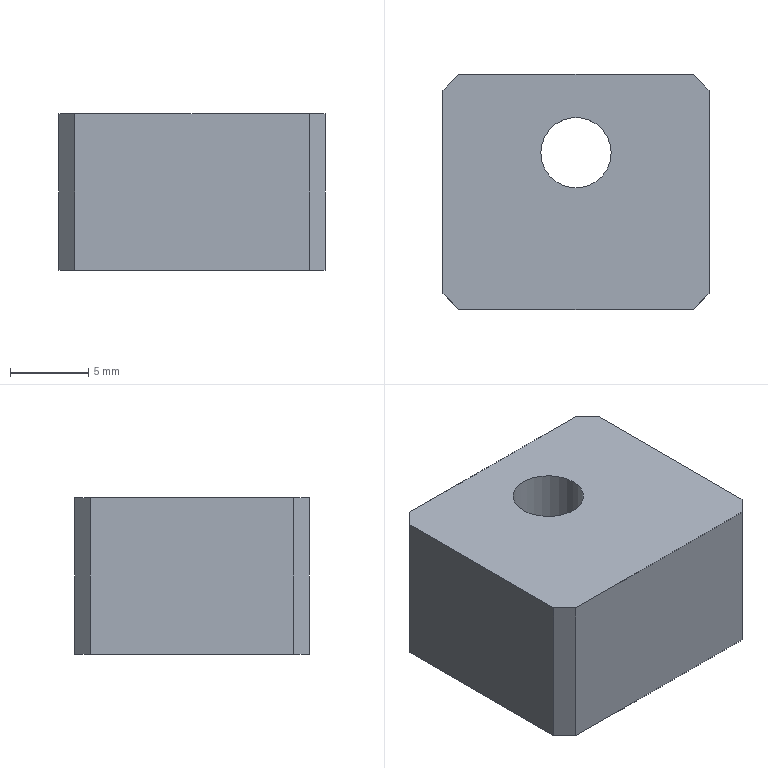Part | STEP file | 1_id906_x_t | 1 solid | 13 faces | box 17 x 15 x 10 mm | volume 2199 mm3 | plane 11 | cylinder 2 | commonest cylinder face diameters 4.5 x1 8 x1
STEP:
#1=CARTESIAN_POINT('',(0.,0.,0.));
#2=DIRECTION('',(0.,0.,1.));
#3=DIRECTION('',(1.,0.,0.));
#4=AXIS2_PLACEMENT_3D('',#1,#2,#3);
#5=CARTESIAN_POINT('',(628.275,227.376,-49.278));
#6=VERTEX_POINT('',#5);
#7=CARTESIAN_POINT('',(628.275,227.376,-59.278));
#8=VERTEX_POINT('',#7);
#9=CARTESIAN_POINT('',(628.275,227.376,-49.278));
#10=DIRECTION('',(0.,0.,-1.));
#11=VECTOR('',#10,1.);
#12=LINE('',#9,#11);
#13=CARTESIAN_POINT('',(627.275,228.376,-49.278));
#14=DIRECTION('',(0.7071,0.7071,0.));
#15=DIRECTION('',(0.,0.,1.));
#16=AXIS2_PLACEMENT_3D('',#13,#14,#15);
#17=PLANE('',#16);
#18=CARTESIAN_POINT('',(0.,1.414));
#19=DIRECTION('',(-1.,0.));
#20=VECTOR('',#19,1.);
#21=LINE('',#18,#20);
#22=(GEOMETRIC_REPRESENTATION_CONTEXT(2)PARAMETRIC_REPRESENTATION_CONTEXT()REPRESENTATION_CONTEXT('',''));
#23=DEFINITIONAL_REPRESENTATION('',(#21),#22);
#24=PCURVE('',#17,#23);
#25=CARTESIAN_POINT('',(643.275,227.376,-49.278));
#26=DIRECTION('',(0.,1.,0.));
#27=DIRECTION('',(-1.,0.,0.));
#28=AXIS2_PLACEMENT_3D('',#25,#26,#27);
#29=PLANE('',#28);
#30=CARTESIAN_POINT('',(15.,0.));
#31=DIRECTION('',(0.,-1.));
#32=VECTOR('',#31,1.);
#33=LINE('',#30,#32);
#34=(GEOMETRIC_REPRESENTATION_CONTEXT(2)PARAMETRIC_REPRESENTATION_CONTEXT()REPRESENTATION_CONTEXT('',''));
#35=DEFINITIONAL_REPRESENTATION('',(#33),#34);
#36=PCURVE('',#29,#35);
#37=SURFACE_CURVE('',#12,(#24,#36),.PCURVE_S1.);
#38=EDGE_CURVE('',#6,#8,#37,.T.);
#39=ORIENTED_EDGE('',*,*,#38,.F.);
#40=CARTESIAN_POINT('',(627.275,228.376,-49.278));
#41=VERTEX_POINT('',#40);
#42=CARTESIAN_POINT('',(627.275,228.376,-49.278));
#43=DIRECTION('',(0.7071,-0.7071,0.));
#44=VECTOR('',#43,1.);
#45=LINE('',#42,#44);
#46=CARTESIAN_POINT('',(0.,0.));
#47=DIRECTION('',(0.,1.));
#48=VECTOR('',#47,1.);
#49=LINE('',#46,#48);
#50=(GEOMETRIC_REPRESENTATION_CONTEXT(2)PARAMETRIC_REPRESENTATION_CONTEXT()REPRESENTATION_CONTEXT('',''));
#51=DEFINITIONAL_REPRESENTATION('',(#49),#50);
#52=PCURVE('',#17,#51);
#53=CARTESIAN_POINT('',(628.275,242.376,-49.278));
#54=DIRECTION('',(0.,0.,1.));
#55=DIRECTION('',(-1.,0.,0.));
#56=AXIS2_PLACEMENT_3D('',#53,#54,#55);
#57=PLANE('',#56);
#58=CARTESIAN_POINT('',(1.,14.));
#59=DIRECTION('',(-0.7071,0.7071));
#60=VECTOR('',#59,1.);
#61=LINE('',#58,#60);
#62=(GEOMETRIC_REPRESENTATION_CONTEXT(2)PARAMETRIC_REPRESENTATION_CONTEXT()REPRESENTATION_CONTEXT('',''));
#63=DEFINITIONAL_REPRESENTATION('',(#61),#62);
#64=PCURVE('',#57,#63);
#65=SURFACE_CURVE('',#45,(#52,#64),.PCURVE_S1.);
#66=EDGE_CURVE('',#41,#6,#65,.T.);
#67=ORIENTED_EDGE('',*,*,#66,.F.);
#68=CARTESIAN_POINT('',(627.275,228.376,-59.278));
#69=VERTEX_POINT('',#68);
#70=CARTESIAN_POINT('',(627.275,228.376,-59.278));
#71=DIRECTION('',(0.,0.,1.));
#72=VECTOR('',#71,1.);
#73=LINE('',#70,#72);
#74=CARTESIAN_POINT('',(-10.,0.));
#75=DIRECTION('',(1.,0.));
#76=VECTOR('',#75,1.);
#77=LINE('',#74,#76);
#78=(GEOMETRIC_REPRESENTATION_CONTEXT(2)PARAMETRIC_REPRESENTATION_CONTEXT()REPRESENTATION_CONTEXT('',''));
#79=DEFINITIONAL_REPRESENTATION('',(#77),#78);
#80=PCURVE('',#17,#79);
#81=CARTESIAN_POINT('',(627.275,227.376,-49.278));
#82=DIRECTION('',(1.,0.,0.));
#83=DIRECTION('',(0.,-1.,0.));
#84=AXIS2_PLACEMENT_3D('',#81,#82,#83);
#85=PLANE('',#84);
#86=CARTESIAN_POINT('',(-1.,10.));
#87=DIRECTION('',(0.,-1.));
#88=VECTOR('',#87,1.);
#89=LINE('',#86,#88);
#90=(GEOMETRIC_REPRESENTATION_CONTEXT(2)PARAMETRIC_REPRESENTATION_CONTEXT()REPRESENTATION_CONTEXT('',''));
#91=DEFINITIONAL_REPRESENTATION('',(#89),#90);
#92=PCURVE('',#85,#91);
#93=SURFACE_CURVE('',#73,(#80,#92),.PCURVE_S1.);
#94=EDGE_CURVE('',#69,#41,#93,.T.);
#95=ORIENTED_EDGE('',*,*,#94,.F.);
#96=CARTESIAN_POINT('',(628.275,227.376,-59.278));
#97=DIRECTION('',(-0.7071,0.7071,0.));
#98=VECTOR('',#97,1.);
#99=LINE('',#96,#98);
#100=CARTESIAN_POINT('',(-10.,1.414));
#101=DIRECTION('',(0.,-1.));
#102=VECTOR('',#101,1.);
#103=LINE('',#100,#102);
#104=(GEOMETRIC_REPRESENTATION_CONTEXT(2)PARAMETRIC_REPRESENTATION_CONTEXT()REPRESENTATION_CONTEXT('',''));
#105=DEFINITIONAL_REPRESENTATION('',(#103),#104);
#106=PCURVE('',#17,#105);
#107=CARTESIAN_POINT('',(628.275,242.376,-59.278));
#108=DIRECTION('',(0.,0.,1.));
#109=DIRECTION('',(-1.,0.,0.));
#110=AXIS2_PLACEMENT_3D('',#107,#108,#109);
#111=PLANE('',#110);
#112=CARTESIAN_POINT('',(0.,15.));
#113=DIRECTION('',(0.7071,-0.7071));
#114=VECTOR('',#113,1.);
#115=LINE('',#112,#114);
#116=(GEOMETRIC_REPRESENTATION_CONTEXT(2)PARAMETRIC_REPRESENTATION_CONTEXT()REPRESENTATION_CONTEXT('',''));
#117=DEFINITIONAL_REPRESENTATION('',(#115),#116);
#118=PCURVE('',#111,#117);
#119=SURFACE_CURVE('',#99,(#106,#118),.PCURVE_S1.);
#120=EDGE_CURVE('',#8,#69,#119,.T.);
#121=ORIENTED_EDGE('',*,*,#120,.F.);
#122=EDGE_LOOP('',(#39,#67,#95,#121));
#123=FACE_BOUND('',#122,.T.);
#124=ADVANCED_FACE('',(#123),#17,.F.);
#125=CARTESIAN_POINT('',(643.275,227.376,-59.278));
#126=VERTEX_POINT('',#125);
#127=CARTESIAN_POINT('',(628.275,227.376,-59.278));
#128=DIRECTION('',(1.,0.,0.));
#129=VECTOR('',#128,1.);
#130=LINE('',#127,#129);
#131=CARTESIAN_POINT('',(0.,15.));
#132=DIRECTION('',(-1.,0.));
#133=VECTOR('',#132,1.);
#134=LINE('',#131,#133);
#135=(GEOMETRIC_REPRESENTATION_CONTEXT(2)PARAMETRIC_REPRESENTATION_CONTEXT()REPRESENTATION_CONTEXT('',''));
#136=DEFINITIONAL_REPRESENTATION('',(#134),#135);
#137=PCURVE('',#111,#136);
#138=CARTESIAN_POINT('',(15.,-10.));
#139=DIRECTION('',(-1.,0.));
#140=VECTOR('',#139,1.);
#141=LINE('',#138,#140);
#142=(GEOMETRIC_REPRESENTATION_CONTEXT(2)PARAMETRIC_REPRESENTATION_CONTEXT()REPRESENTATION_CONTEXT('',''));
#143=DEFINITIONAL_REPRESENTATION('',(#141),#142);
#144=PCURVE('',#29,#143);
#145=SURFACE_CURVE('',#130,(#137,#144),.PCURVE_S1.);
#146=EDGE_CURVE('',#8,#126,#145,.T.);
#147=ORIENTED_EDGE('',*,*,#146,.F.);
#148=ORIENTED_EDGE('',*,*,#120,.T.);
#149=CARTESIAN_POINT('',(627.275,241.376,-59.278));
#150=VERTEX_POINT('',#149);
#151=CARTESIAN_POINT('',(627.275,241.376,-59.278));
#152=DIRECTION('',(0.,-1.,0.));
#153=VECTOR('',#152,1.);
#154=LINE('',#151,#153);
#155=CARTESIAN_POINT('',(1.,1.));
#156=DIRECTION('',(0.,1.));
#157=VECTOR('',#156,1.);
#158=LINE('',#155,#157);
#159=(GEOMETRIC_REPRESENTATION_CONTEXT(2)PARAMETRIC_REPRESENTATION_CONTEXT()REPRESENTATION_CONTEXT('',''));
#160=DEFINITIONAL_REPRESENTATION('',(#158),#159);
#161=PCURVE('',#111,#160);
#162=CARTESIAN_POINT('',(-14.,10.));
#163=DIRECTION('',(1.,0.));
#164=VECTOR('',#163,1.);
#165=LINE('',#162,#164);
#166=(GEOMETRIC_REPRESENTATION_CONTEXT(2)PARAMETRIC_REPRESENTATION_CONTEXT()REPRESENTATION_CONTEXT('',''));
#167=DEFINITIONAL_REPRESENTATION('',(#165),#166);
#168=PCURVE('',#85,#167);
#169=SURFACE_CURVE('',#154,(#161,#168),.PCURVE_S1.);
#170=EDGE_CURVE('',#150,#69,#169,.T.);
#171=ORIENTED_EDGE('',*,*,#170,.F.);
#172=CARTESIAN_POINT('',(628.275,242.376,-59.278));
#173=VERTEX_POINT('',#172);
#174=CARTESIAN_POINT('',(627.275,241.376,-59.278));
#175=DIRECTION('',(0.7071,0.7071,0.));
#176=VECTOR('',#175,1.);
#177=LINE('',#174,#176);
#178=CARTESIAN_POINT('',(1.,1.));
#179=DIRECTION('',(-0.7071,-0.7071));
#180=VECTOR('',#179,1.);
#181=LINE('',#178,#180);
#182=(GEOMETRIC_REPRESENTATION_CONTEXT(2)PARAMETRIC_REPRESENTATION_CONTEXT()REPRESENTATION_CONTEXT('',''));
#183=DEFINITIONAL_REPRESENTATION('',(#181),#182);
#184=PCURVE('',#111,#183);
#185=CARTESIAN_POINT('',(627.275,241.376,-49.278));
#186=DIRECTION('',(0.7071,-0.7071,0.));
#187=DIRECTION('',(0.7071,0.7071,0.));
#188=AXIS2_PLACEMENT_3D('',#185,#186,#187);
#189=PLANE('',#188);
#190=CARTESIAN_POINT('',(0.,-10.));
#191=DIRECTION('',(1.,0.));
#192=VECTOR('',#191,1.);
#193=LINE('',#190,#192);
#194=(GEOMETRIC_REPRESENTATION_CONTEXT(2)PARAMETRIC_REPRESENTATION_CONTEXT()REPRESENTATION_CONTEXT('',''));
#195=DEFINITIONAL_REPRESENTATION('',(#193),#194);
#196=PCURVE('',#189,#195);
#197=SURFACE_CURVE('',#177,(#184,#196),.PCURVE_S1.);
#198=EDGE_CURVE('',#150,#173,#197,.T.);
#199=ORIENTED_EDGE('',*,*,#198,.T.);
#200=CARTESIAN_POINT('',(643.275,242.376,-59.278));
#201=VERTEX_POINT('',#200);
#202=CARTESIAN_POINT('',(643.275,242.376,-59.278));
#203=DIRECTION('',(-1.,0.,0.));
#204=VECTOR('',#203,1.);
#205=LINE('',#202,#204);
#206=CARTESIAN_POINT('',(-15.,0.));
#207=DIRECTION('',(1.,0.));
#208=VECTOR('',#207,1.);
#209=LINE('',#206,#208);
#210=(GEOMETRIC_REPRESENTATION_CONTEXT(2)PARAMETRIC_REPRESENTATION_CONTEXT()REPRESENTATION_CONTEXT('',''));
#211=DEFINITIONAL_REPRESENTATION('',(#209),#210);
#212=PCURVE('',#111,#211);
#213=CARTESIAN_POINT('',(628.275,242.376,-49.278));
#214=DIRECTION('',(0.,-1.,0.));
#215=DIRECTION('',(0.,0.,1.));
#216=AXIS2_PLACEMENT_3D('',#213,#214,#215);
#217=PLANE('',#216);
#218=CARTESIAN_POINT('',(-10.,-15.));
#219=DIRECTION('',(0.,1.));
#220=VECTOR('',#219,1.);
#221=LINE('',#218,#220);
#222=(GEOMETRIC_REPRESENTATION_CONTEXT(2)PARAMETRIC_REPRESENTATION_CONTEXT()REPRESENTATION_CONTEXT('',''));
#223=DEFINITIONAL_REPRESENTATION('',(#221),#222);
#224=PCURVE('',#217,#223);
#225=SURFACE_CURVE('',#205,(#212,#224),.PCURVE_S1.);
#226=EDGE_CURVE('',#201,#173,#225,.T.);
#227=ORIENTED_EDGE('',*,*,#226,.F.);
#228=CARTESIAN_POINT('',(644.275,241.376,-59.278));
#229=VERTEX_POINT('',#228);
#230=CARTESIAN_POINT('',(643.275,242.376,-59.278));
#231=DIRECTION('',(0.7071,-0.7071,0.));
#232=VECTOR('',#231,1.);
#233=LINE('',#230,#232);
#234=CARTESIAN_POINT('',(-15.,0.));
#235=DIRECTION('',(-0.7071,0.7071));
#236=VECTOR('',#235,1.);
#237=LINE('',#234,#236);
#238=(GEOMETRIC_REPRESENTATION_CONTEXT(2)PARAMETRIC_REPRESENTATION_CONTEXT()REPRESENTATION_CONTEXT('',''));
#239=DEFINITIONAL_REPRESENTATION('',(#237),#238);
#240=PCURVE('',#111,#239);
#241=CARTESIAN_POINT('',(644.275,241.376,-49.278));
#242=DIRECTION('',(-0.7071,-0.7071,0.));
#243=DIRECTION('',(0.7071,-0.7071,0.));
#244=AXIS2_PLACEMENT_3D('',#241,#242,#243);
#245=PLANE('',#244);
#246=CARTESIAN_POINT('',(-1.414,-10.));
#247=DIRECTION('',(1.,0.));
#248=VECTOR('',#247,1.);
#249=LINE('',#246,#248);
#250=(GEOMETRIC_REPRESENTATION_CONTEXT(2)PARAMETRIC_REPRESENTATION_CONTEXT()REPRESENTATION_CONTEXT('',''));
#251=DEFINITIONAL_REPRESENTATION('',(#249),#250);
#252=PCURVE('',#245,#251);
#253=SURFACE_CURVE('',#233,(#240,#252),.PCURVE_S1.);
#254=EDGE_CURVE('',#201,#229,#253,.T.);
#255=ORIENTED_EDGE('',*,*,#254,.T.);
#256=CARTESIAN_POINT('',(644.275,228.376,-59.278));
#257=VERTEX_POINT('',#256);
#258=CARTESIAN_POINT('',(644.275,228.376,-59.278));
#259=DIRECTION('',(0.,1.,0.));
#260=VECTOR('',#259,1.);
#261=LINE('',#258,#260);
#262=CARTESIAN_POINT('',(-16.,14.));
#263=DIRECTION('',(0.,-1.));
#264=VECTOR('',#263,1.);
#265=LINE('',#262,#264);
#266=(GEOMETRIC_REPRESENTATION_CONTEXT(2)PARAMETRIC_REPRESENTATION_CONTEXT()REPRESENTATION_CONTEXT('',''));
#267=DEFINITIONAL_REPRESENTATION('',(#265),#266);
#268=PCURVE('',#111,#267);
#269=CARTESIAN_POINT('',(644.275,242.376,-49.278));
#270=DIRECTION('',(-1.,0.,0.));
#271=DIRECTION('',(0.,0.,-1.));
#272=AXIS2_PLACEMENT_3D('',#269,#270,#271);
#273=PLANE('',#272);
#274=CARTESIAN_POINT('',(10.,14.));
#275=DIRECTION('',(0.,-1.));
#276=VECTOR('',#275,1.);
#277=LINE('',#274,#276);
#278=(GEOMETRIC_REPRESENTATION_CONTEXT(2)PARAMETRIC_REPRESENTATION_CONTEXT()REPRESENTATION_CONTEXT('',''));
#279=DEFINITIONAL_REPRESENTATION('',(#277),#278);
#280=PCURVE('',#273,#279);
#281=SURFACE_CURVE('',#261,(#268,#280),.PCURVE_S1.);
#282=EDGE_CURVE('',#257,#229,#281,.T.);
#283=ORIENTED_EDGE('',*,*,#282,.F.);
#284=CARTESIAN_POINT('',(644.275,228.376,-59.278));
#285=DIRECTION('',(-0.7071,-0.7071,0.));
#286=VECTOR('',#285,1.);
#287=LINE('',#284,#286);
#288=CARTESIAN_POINT('',(-16.,14.));
#289=DIRECTION('',(0.7071,0.7071));
#290=VECTOR('',#289,1.);
#291=LINE('',#288,#290);
#292=(GEOMETRIC_REPRESENTATION_CONTEXT(2)PARAMETRIC_REPRESENTATION_CONTEXT()REPRESENTATION_CONTEXT('',''));
#293=DEFINITIONAL_REPRESENTATION('',(#291),#292);
#294=PCURVE('',#111,#293);
#295=CARTESIAN_POINT('',(643.275,227.376,-49.278));
#296=DIRECTION('',(-0.7071,0.7071,0.));
#297=DIRECTION('',(0.,0.,-1.));
#298=AXIS2_PLACEMENT_3D('',#295,#296,#297);
#299=PLANE('',#298);
#300=CARTESIAN_POINT('',(10.,-1.414));
#301=DIRECTION('',(0.,1.));
#302=VECTOR('',#301,1.);
#303=LINE('',#300,#302);
#304=(GEOMETRIC_REPRESENTATION_CONTEXT(2)PARAMETRIC_REPRESENTATION_CONTEXT()REPRESENTATION_CONTEXT('',''));
#305=DEFINITIONAL_REPRESENTATION('',(#303),#304);
#306=PCURVE('',#299,#305);
#307=SURFACE_CURVE('',#287,(#294,#306),.PCURVE_S1.);
#308=EDGE_CURVE('',#257,#126,#307,.T.);
#309=ORIENTED_EDGE('',*,*,#308,.T.);
#310=EDGE_LOOP('',(#147,#148,#171,#199,#227,#255,#283,#309));
#311=FACE_BOUND('',#310,.T.);
#312=CARTESIAN_POINT('',(631.775,237.376,-59.278));
#313=VERTEX_POINT('',#312);
#314=CARTESIAN_POINT('',(635.775,237.376,-59.278));
#315=DIRECTION('',(0.,0.,1.));
#316=DIRECTION('',(-1.,0.,0.));
#317=AXIS2_PLACEMENT_3D('',#314,#315,#316);
#318=CIRCLE('',#317,4.);
#319=CARTESIAN_POINT('',(-7.5,5.));
#320=DIRECTION('',(1.,0.));
#321=AXIS2_PLACEMENT_2D('',#319,#320);
#322=CIRCLE('',#321,4.);
#323=(GEOMETRIC_REPRESENTATION_CONTEXT(2)PARAMETRIC_REPRESENTATION_CONTEXT()REPRESENTATION_CONTEXT('',''));
#324=DEFINITIONAL_REPRESENTATION('',(#322),#323);
#325=PCURVE('',#111,#324);
#326=CARTESIAN_POINT('',(635.775,237.376,-54.278));
#327=DIRECTION('',(0.,0.,1.));
#328=DIRECTION('',(1.,0.,0.));
#329=AXIS2_PLACEMENT_3D('',#326,#327,#328);
#330=CYLINDRICAL_SURFACE('',#329,4.);
#331=CARTESIAN_POINT('',(3.142,-5.));
#332=DIRECTION('',(1.,0.));
#333=VECTOR('',#332,1.);
#334=LINE('',#331,#333);
#335=(GEOMETRIC_REPRESENTATION_CONTEXT(2)PARAMETRIC_REPRESENTATION_CONTEXT()REPRESENTATION_CONTEXT('',''));
#336=DEFINITIONAL_REPRESENTATION('',(#334),#335);
#337=PCURVE('',#330,#336);
#338=SURFACE_CURVE('',#318,(#325,#337),.PCURVE_S1.);
#339=EDGE_CURVE('',#313,#313,#338,.T.);
#340=ORIENTED_EDGE('',*,*,#339,.T.);
#341=EDGE_LOOP('',(#340));
#342=FACE_BOUND('',#341,.T.);
#343=ADVANCED_FACE('',(#311,#342),#111,.F.);
#344=CARTESIAN_POINT('',(643.275,227.376,-49.278));
#345=VERTEX_POINT('',#344);
#346=CARTESIAN_POINT('',(643.275,227.376,-59.278));
#347=DIRECTION('',(0.,0.,1.));
#348=VECTOR('',#347,1.);
#349=LINE('',#346,#348);
#350=CARTESIAN_POINT('',(10.,0.));
#351=DIRECTION('',(-1.,0.));
#352=VECTOR('',#351,1.);
#353=LINE('',#350,#352);
#354=(GEOMETRIC_REPRESENTATION_CONTEXT(2)PARAMETRIC_REPRESENTATION_CONTEXT()REPRESENTATION_CONTEXT('',''));
#355=DEFINITIONAL_REPRESENTATION('',(#353),#354);
#356=PCURVE('',#299,#355);
#357=CARTESIAN_POINT('',(0.,-10.));
#358=DIRECTION('',(0.,1.));
#359=VECTOR('',#358,1.);
#360=LINE('',#357,#359);
#361=(GEOMETRIC_REPRESENTATION_CONTEXT(2)PARAMETRIC_REPRESENTATION_CONTEXT()REPRESENTATION_CONTEXT('',''));
#362=DEFINITIONAL_REPRESENTATION('',(#360),#361);
#363=PCURVE('',#29,#362);
#364=SURFACE_CURVE('',#349,(#356,#363),.PCURVE_S1.);
#365=EDGE_CURVE('',#126,#345,#364,.T.);
#366=ORIENTED_EDGE('',*,*,#365,.F.);
#367=ORIENTED_EDGE('',*,*,#308,.F.);
#368=CARTESIAN_POINT('',(644.275,228.376,-49.278));
#369=VERTEX_POINT('',#368);
#370=CARTESIAN_POINT('',(644.275,228.376,-49.278));
#371=DIRECTION('',(0.,0.,-1.));
#372=VECTOR('',#371,1.);
#373=LINE('',#370,#372);
#374=CARTESIAN_POINT('',(0.,-1.414));
#375=DIRECTION('',(1.,0.));
#376=VECTOR('',#375,1.);
#377=LINE('',#374,#376);
#378=(GEOMETRIC_REPRESENTATION_CONTEXT(2)PARAMETRIC_REPRESENTATION_CONTEXT()REPRESENTATION_CONTEXT('',''));
#379=DEFINITIONAL_REPRESENTATION('',(#377),#378);
#380=PCURVE('',#299,#379);
#381=CARTESIAN_POINT('',(0.,14.));
#382=DIRECTION('',(1.,0.));
#383=VECTOR('',#382,1.);
#384=LINE('',#381,#383);
#385=(GEOMETRIC_REPRESENTATION_CONTEXT(2)PARAMETRIC_REPRESENTATION_CONTEXT()REPRESENTATION_CONTEXT('',''));
#386=DEFINITIONAL_REPRESENTATION('',(#384),#385);
#387=PCURVE('',#273,#386);
#388=SURFACE_CURVE('',#373,(#380,#387),.PCURVE_S1.);
#389=EDGE_CURVE('',#369,#257,#388,.T.);
#390=ORIENTED_EDGE('',*,*,#389,.F.);
#391=CARTESIAN_POINT('',(643.275,227.376,-49.278));
#392=DIRECTION('',(0.7071,0.7071,0.));
#393=VECTOR('',#392,1.);
#394=LINE('',#391,#393);
#395=CARTESIAN_POINT('',(0.,0.));
#396=DIRECTION('',(0.,-1.));
#397=VECTOR('',#396,1.);
#398=LINE('',#395,#397);
#399=(GEOMETRIC_REPRESENTATION_CONTEXT(2)PARAMETRIC_REPRESENTATION_CONTEXT()REPRESENTATION_CONTEXT('',''));
#400=DEFINITIONAL_REPRESENTATION('',(#398),#399);
#401=PCURVE('',#299,#400);
#402=CARTESIAN_POINT('',(-15.,15.));
#403=DIRECTION('',(-0.7071,-0.7071));
#404=VECTOR('',#403,1.);
#405=LINE('',#402,#404);
#406=(GEOMETRIC_REPRESENTATION_CONTEXT(2)PARAMETRIC_REPRESENTATION_CONTEXT()REPRESENTATION_CONTEXT('',''));
#407=DEFINITIONAL_REPRESENTATION('',(#405),#406);
#408=PCURVE('',#57,#407);
#409=SURFACE_CURVE('',#394,(#401,#408),.PCURVE_S1.);
#410=EDGE_CURVE('',#345,#369,#409,.T.);
#411=ORIENTED_EDGE('',*,*,#410,.F.);
#412=EDGE_LOOP('',(#366,#367,#390,#411));
#413=FACE_BOUND('',#412,.T.);
#414=ADVANCED_FACE('',(#413),#299,.F.);
#415=CARTESIAN_POINT('',(628.275,227.376,-49.278));
#416=DIRECTION('',(1.,0.,0.));
#417=VECTOR('',#416,1.);
#418=LINE('',#415,#417);
#419=CARTESIAN_POINT('',(0.,15.));
#420=DIRECTION('',(-1.,0.));
#421=VECTOR('',#420,1.);
#422=LINE('',#419,#421);
#423=(GEOMETRIC_REPRESENTATION_CONTEXT(2)PARAMETRIC_REPRESENTATION_CONTEXT()REPRESENTATION_CONTEXT('',''));
#424=DEFINITIONAL_REPRESENTATION('',(#422),#423);
#425=PCURVE('',#57,#424);
#426=CARTESIAN_POINT('',(15.,0.));
#427=DIRECTION('',(-1.,0.));
#428=VECTOR('',#427,1.);
#429=LINE('',#426,#428);
#430=(GEOMETRIC_REPRESENTATION_CONTEXT(2)PARAMETRIC_REPRESENTATION_CONTEXT()REPRESENTATION_CONTEXT('',''));
#431=DEFINITIONAL_REPRESENTATION('',(#429),#430);
#432=PCURVE('',#29,#431);
#433=SURFACE_CURVE('',#418,(#425,#432),.PCURVE_S1.);
#434=EDGE_CURVE('',#6,#345,#433,.T.);
#435=ORIENTED_EDGE('',*,*,#434,.T.);
#436=ORIENTED_EDGE('',*,*,#410,.T.);
#437=CARTESIAN_POINT('',(644.275,241.376,-49.278));
#438=VERTEX_POINT('',#437);
#439=CARTESIAN_POINT('',(644.275,228.376,-49.278));
#440=DIRECTION('',(0.,1.,0.));
#441=VECTOR('',#440,1.);
#442=LINE('',#439,#441);
#443=CARTESIAN_POINT('',(-16.,14.));
#444=DIRECTION('',(0.,-1.));
#445=VECTOR('',#444,1.);
#446=LINE('',#443,#445);
#447=(GEOMETRIC_REPRESENTATION_CONTEXT(2)PARAMETRIC_REPRESENTATION_CONTEXT()REPRESENTATION_CONTEXT('',''));
#448=DEFINITIONAL_REPRESENTATION('',(#446),#447);
#449=PCURVE('',#57,#448);
#450=CARTESIAN_POINT('',(0.,14.));
#451=DIRECTION('',(0.,-1.));
#452=VECTOR('',#451,1.);
#453=LINE('',#450,#452);
#454=(GEOMETRIC_REPRESENTATION_CONTEXT(2)PARAMETRIC_REPRESENTATION_CONTEXT()REPRESENTATION_CONTEXT('',''));
#455=DEFINITIONAL_REPRESENTATION('',(#453),#454);
#456=PCURVE('',#273,#455);
#457=SURFACE_CURVE('',#442,(#449,#456),.PCURVE_S1.);
#458=EDGE_CURVE('',#369,#438,#457,.T.);
#459=ORIENTED_EDGE('',*,*,#458,.T.);
#460=CARTESIAN_POINT('',(643.275,242.376,-49.278));
#461=VERTEX_POINT('',#460);
#462=CARTESIAN_POINT('',(644.275,241.376,-49.278));
#463=DIRECTION('',(-0.7071,0.7071,0.));
#464=VECTOR('',#463,1.);
#465=LINE('',#462,#464);
#466=CARTESIAN_POINT('',(-16.,1.));
#467=DIRECTION('',(0.7071,-0.7071));
#468=VECTOR('',#467,1.);
#469=LINE('',#466,#468);
#470=(GEOMETRIC_REPRESENTATION_CONTEXT(2)PARAMETRIC_REPRESENTATION_CONTEXT()REPRESENTATION_CONTEXT('',''));
#471=DEFINITIONAL_REPRESENTATION('',(#469),#470);
#472=PCURVE('',#57,#471);
#473=CARTESIAN_POINT('',(0.,0.));
#474=DIRECTION('',(-1.,0.));
#475=VECTOR('',#474,1.);
#476=LINE('',#473,#475);
#477=(GEOMETRIC_REPRESENTATION_CONTEXT(2)PARAMETRIC_REPRESENTATION_CONTEXT()REPRESENTATION_CONTEXT('',''));
#478=DEFINITIONAL_REPRESENTATION('',(#476),#477);
#479=PCURVE('',#245,#478);
#480=SURFACE_CURVE('',#465,(#472,#479),.PCURVE_S1.);
#481=EDGE_CURVE('',#438,#461,#480,.T.);
#482=ORIENTED_EDGE('',*,*,#481,.T.);
#483=CARTESIAN_POINT('',(628.275,242.376,-49.278));
#484=VERTEX_POINT('',#483);
#485=CARTESIAN_POINT('',(643.275,242.376,-49.278));
#486=DIRECTION('',(-1.,0.,0.));
#487=VECTOR('',#486,1.);
#488=LINE('',#485,#487);
#489=CARTESIAN_POINT('',(-15.,0.));
#490=DIRECTION('',(1.,0.));
#491=VECTOR('',#490,1.);
#492=LINE('',#489,#491);
#493=(GEOMETRIC_REPRESENTATION_CONTEXT(2)PARAMETRIC_REPRESENTATION_CONTEXT()REPRESENTATION_CONTEXT('',''));
#494=DEFINITIONAL_REPRESENTATION('',(#492),#493);
#495=PCURVE('',#57,#494);
#496=CARTESIAN_POINT('',(0.,-15.));
#497=DIRECTION('',(0.,1.));
#498=VECTOR('',#497,1.);
#499=LINE('',#496,#498);
#500=(GEOMETRIC_REPRESENTATION_CONTEXT(2)PARAMETRIC_REPRESENTATION_CONTEXT()REPRESENTATION_CONTEXT('',''));
#501=DEFINITIONAL_REPRESENTATION('',(#499),#500);
#502=PCURVE('',#217,#501);
#503=SURFACE_CURVE('',#488,(#495,#502),.PCURVE_S1.);
#504=EDGE_CURVE('',#461,#484,#503,.T.);
#505=ORIENTED_EDGE('',*,*,#504,.T.);
#506=CARTESIAN_POINT('',(627.275,241.376,-49.278));
#507=VERTEX_POINT('',#506);
#508=CARTESIAN_POINT('',(628.275,242.376,-49.278));
#509=DIRECTION('',(-0.7071,-0.7071,0.));
#510=VECTOR('',#509,1.);
#511=LINE('',#508,#510);
#512=CARTESIAN_POINT('',(0.,0.));
#513=DIRECTION('',(0.7071,0.7071));
#514=VECTOR('',#513,1.);
#515=LINE('',#512,#514);
#516=(GEOMETRIC_REPRESENTATION_CONTEXT(2)PARAMETRIC_REPRESENTATION_CONTEXT()REPRESENTATION_CONTEXT('',''));
#517=DEFINITIONAL_REPRESENTATION('',(#515),#516);
#518=PCURVE('',#57,#517);
#519=CARTESIAN_POINT('',(1.414,0.));
#520=DIRECTION('',(-1.,0.));
#521=VECTOR('',#520,1.);
#522=LINE('',#519,#521);
#523=(GEOMETRIC_REPRESENTATION_CONTEXT(2)PARAMETRIC_REPRESENTATION_CONTEXT()REPRESENTATION_CONTEXT('',''));
#524=DEFINITIONAL_REPRESENTATION('',(#522),#523);
#525=PCURVE('',#189,#524);
#526=SURFACE_CURVE('',#511,(#518,#525),.PCURVE_S1.);
#527=EDGE_CURVE('',#484,#507,#526,.T.);
#528=ORIENTED_EDGE('',*,*,#527,.T.);
#529=CARTESIAN_POINT('',(627.275,241.376,-49.278));
#530=DIRECTION('',(0.,-1.,0.));
#531=VECTOR('',#530,1.);
#532=LINE('',#529,#531);
#533=CARTESIAN_POINT('',(1.,1.));
#534=DIRECTION('',(0.,1.));
#535=VECTOR('',#534,1.);
#536=LINE('',#533,#535);
#537=(GEOMETRIC_REPRESENTATION_CONTEXT(2)PARAMETRIC_REPRESENTATION_CONTEXT()REPRESENTATION_CONTEXT('',''));
#538=DEFINITIONAL_REPRESENTATION('',(#536),#537);
#539=PCURVE('',#57,#538);
#540=CARTESIAN_POINT('',(-14.,0.));
#541=DIRECTION('',(1.,0.));
#542=VECTOR('',#541,1.);
#543=LINE('',#540,#542);
#544=(GEOMETRIC_REPRESENTATION_CONTEXT(2)PARAMETRIC_REPRESENTATION_CONTEXT()REPRESENTATION_CONTEXT('',''));
#545=DEFINITIONAL_REPRESENTATION('',(#543),#544);
#546=PCURVE('',#85,#545);
#547=SURFACE_CURVE('',#532,(#539,#546),.PCURVE_S1.);
#548=EDGE_CURVE('',#507,#41,#547,.T.);
#549=ORIENTED_EDGE('',*,*,#548,.T.);
#550=ORIENTED_EDGE('',*,*,#66,.T.);
#551=EDGE_LOOP('',(#435,#436,#459,#482,#505,#528,#549,#550));
#552=FACE_BOUND('',#551,.T.);
#553=CARTESIAN_POINT('',(638.025,237.376,-49.278));
#554=VERTEX_POINT('',#553);
#555=CARTESIAN_POINT('',(635.775,237.376,-49.278));
#556=DIRECTION('',(0.,0.,-1.));
#557=DIRECTION('',(1.,0.,0.));
#558=AXIS2_PLACEMENT_3D('',#555,#556,#557);
#559=CIRCLE('',#558,2.25);
#560=CARTESIAN_POINT('',(-9.75,5.));
#561=CARTESIAN_POINT('',(-9.75,8.897));
#562=CARTESIAN_POINT('',(-6.375,6.949));
#563=CARTESIAN_POINT('',(-3.,5.));
#564=CARTESIAN_POINT('',(-6.375,3.051));
#565=CARTESIAN_POINT('',(-9.75,1.103));
#566=CARTESIAN_POINT('',(-9.75,5.));
#567=(BOUNDED_CURVE()B_SPLINE_CURVE(2,(#560,#561,#562,#563,#564,#565,#566),.UNSPECIFIED.,.T.,.F.)B_SPLINE_CURVE_WITH_KNOTS((1,2,2,2,2,1),(-2.094,0.,2.094,4.189,6.283,8.378),.UNSPECIFIED.)CURVE()GEOMETRIC_REPRESENTATION_ITEM()RATIONAL_B_SPLINE_CURVE((1.,0.5,1.,0.5,1.,0.5,1.))REPRESENTATION_ITEM(''));
#568=(GEOMETRIC_REPRESENTATION_CONTEXT(2)PARAMETRIC_REPRESENTATION_CONTEXT()REPRESENTATION_CONTEXT('',''));
#569=DEFINITIONAL_REPRESENTATION('',(#567),#568);
#570=PCURVE('',#57,#569);
#571=CARTESIAN_POINT('',(635.775,237.376,-47.028));
#572=DIRECTION('',(0.,0.,1.));
#573=DIRECTION('',(1.,0.,0.));
#574=AXIS2_PLACEMENT_3D('',#571,#572,#573);
#575=CYLINDRICAL_SURFACE('',#574,2.25);
#576=CARTESIAN_POINT('',(6.283,-2.25));
#577=DIRECTION('',(-1.,0.));
#578=VECTOR('',#577,1.);
#579=LINE('',#576,#578);
#580=(GEOMETRIC_REPRESENTATION_CONTEXT(2)PARAMETRIC_REPRESENTATION_CONTEXT()REPRESENTATION_CONTEXT('',''));
#581=DEFINITIONAL_REPRESENTATION('',(#579),#580);
#582=PCURVE('',#575,#581);
#583=SURFACE_CURVE('',#559,(#570,#582),.PCURVE_S1.);
#584=EDGE_CURVE('',#554,#554,#583,.T.);
#585=ORIENTED_EDGE('',*,*,#584,.T.);
#586=EDGE_LOOP('',(#585));
#587=FACE_BOUND('',#586,.T.);
#588=ADVANCED_FACE('',(#552,#587),#57,.T.);
#589=CARTESIAN_POINT('',(627.275,241.376,-59.278));
#590=DIRECTION('',(0.,0.,1.));
#591=VECTOR('',#590,1.);
#592=LINE('',#589,#591);
#593=CARTESIAN_POINT('',(-14.,10.));
#594=DIRECTION('',(0.,-1.));
#595=VECTOR('',#594,1.);
#596=LINE('',#593,#595);
#597=(GEOMETRIC_REPRESENTATION_CONTEXT(2)PARAMETRIC_REPRESENTATION_CONTEXT()REPRESENTATION_CONTEXT('',''));
#598=DEFINITIONAL_REPRESENTATION('',(#596),#597);
#599=PCURVE('',#85,#598);
#600=CARTESIAN_POINT('',(0.,-10.));
#601=DIRECTION('',(0.,1.));
#602=VECTOR('',#601,1.);
#603=LINE('',#600,#602);
#604=(GEOMETRIC_REPRESENTATION_CONTEXT(2)PARAMETRIC_REPRESENTATION_CONTEXT()REPRESENTATION_CONTEXT('',''));
#605=DEFINITIONAL_REPRESENTATION('',(#603),#604);
#606=PCURVE('',#189,#605);
#607=SURFACE_CURVE('',#592,(#599,#606),.PCURVE_S1.);
#608=EDGE_CURVE('',#150,#507,#607,.T.);
#609=ORIENTED_EDGE('',*,*,#608,.F.);
#610=ORIENTED_EDGE('',*,*,#170,.T.);
#611=ORIENTED_EDGE('',*,*,#94,.T.);
#612=ORIENTED_EDGE('',*,*,#548,.F.);
#613=EDGE_LOOP('',(#609,#610,#611,#612));
#614=FACE_BOUND('',#613,.T.);
#615=ADVANCED_FACE('',(#614),#85,.F.);
#616=CARTESIAN_POINT('',(628.275,242.376,-49.278));
#617=DIRECTION('',(0.,0.,-1.));
#618=VECTOR('',#617,1.);
#619=LINE('',#616,#618);
#620=CARTESIAN_POINT('',(1.414,0.));
#621=DIRECTION('',(0.,-1.));
#622=VECTOR('',#621,1.);
#623=LINE('',#620,#622);
#624=(GEOMETRIC_REPRESENTATION_CONTEXT(2)PARAMETRIC_REPRESENTATION_CONTEXT()REPRESENTATION_CONTEXT('',''));
#625=DEFINITIONAL_REPRESENTATION('',(#623),#624);
#626=PCURVE('',#189,#625);
#627=CARTESIAN_POINT('',(0.,0.));
#628=DIRECTION('',(-1.,0.));
#629=VECTOR('',#628,1.);
#630=LINE('',#627,#629);
#631=(GEOMETRIC_REPRESENTATION_CONTEXT(2)PARAMETRIC_REPRESENTATION_CONTEXT()REPRESENTATION_CONTEXT('',''));
#632=DEFINITIONAL_REPRESENTATION('',(#630),#631);
#633=PCURVE('',#217,#632);
#634=SURFACE_CURVE('',#619,(#626,#633),.PCURVE_S1.);
#635=EDGE_CURVE('',#484,#173,#634,.T.);
#636=ORIENTED_EDGE('',*,*,#635,.T.);
#637=ORIENTED_EDGE('',*,*,#198,.F.);
#638=ORIENTED_EDGE('',*,*,#608,.T.);
#639=ORIENTED_EDGE('',*,*,#527,.F.);
#640=EDGE_LOOP('',(#636,#637,#638,#639));
#641=FACE_BOUND('',#640,.T.);
#642=ADVANCED_FACE('',(#641),#189,.F.);
#643=ORIENTED_EDGE('',*,*,#635,.F.);
#644=ORIENTED_EDGE('',*,*,#504,.F.);
#645=CARTESIAN_POINT('',(643.275,242.376,-59.278));
#646=DIRECTION('',(0.,0.,1.));
#647=VECTOR('',#646,1.);
#648=LINE('',#645,#647);
#649=CARTESIAN_POINT('',(-10.,-15.));
#650=DIRECTION('',(1.,0.));
#651=VECTOR('',#650,1.);
#652=LINE('',#649,#651);
#653=(GEOMETRIC_REPRESENTATION_CONTEXT(2)PARAMETRIC_REPRESENTATION_CONTEXT()REPRESENTATION_CONTEXT('',''));
#654=DEFINITIONAL_REPRESENTATION('',(#652),#653);
#655=PCURVE('',#217,#654);
#656=CARTESIAN_POINT('',(-1.414,-10.));
#657=DIRECTION('',(0.,1.));
#658=VECTOR('',#657,1.);
#659=LINE('',#656,#658);
#660=(GEOMETRIC_REPRESENTATION_CONTEXT(2)PARAMETRIC_REPRESENTATION_CONTEXT()REPRESENTATION_CONTEXT('',''));
#661=DEFINITIONAL_REPRESENTATION('',(#659),#660);
#662=PCURVE('',#245,#661);
#663=SURFACE_CURVE('',#648,(#655,#662),.PCURVE_S1.);
#664=EDGE_CURVE('',#201,#461,#663,.T.);
#665=ORIENTED_EDGE('',*,*,#664,.F.);
#666=ORIENTED_EDGE('',*,*,#226,.T.);
#667=EDGE_LOOP('',(#643,#644,#665,#666));
#668=FACE_BOUND('',#667,.T.);
#669=ADVANCED_FACE('',(#668),#217,.F.);
#670=ORIENTED_EDGE('',*,*,#664,.T.);
#671=ORIENTED_EDGE('',*,*,#481,.F.);
#672=CARTESIAN_POINT('',(644.275,241.376,-49.278));
#673=DIRECTION('',(0.,0.,-1.));
#674=VECTOR('',#673,1.);
#675=LINE('',#672,#674);
#676=CARTESIAN_POINT('',(0.,0.));
#677=DIRECTION('',(0.,-1.));
#678=VECTOR('',#677,1.);
#679=LINE('',#676,#678);
#680=(GEOMETRIC_REPRESENTATION_CONTEXT(2)PARAMETRIC_REPRESENTATION_CONTEXT()REPRESENTATION_CONTEXT('',''));
#681=DEFINITIONAL_REPRESENTATION('',(#679),#680);
#682=PCURVE('',#245,#681);
#683=CARTESIAN_POINT('',(0.,1.));
#684=DIRECTION('',(1.,0.));
#685=VECTOR('',#684,1.);
#686=LINE('',#683,#685);
#687=(GEOMETRIC_REPRESENTATION_CONTEXT(2)PARAMETRIC_REPRESENTATION_CONTEXT()REPRESENTATION_CONTEXT('',''));
#688=DEFINITIONAL_REPRESENTATION('',(#686),#687);
#689=PCURVE('',#273,#688);
#690=SURFACE_CURVE('',#675,(#682,#689),.PCURVE_S1.);
#691=EDGE_CURVE('',#438,#229,#690,.T.);
#692=ORIENTED_EDGE('',*,*,#691,.T.);
#693=ORIENTED_EDGE('',*,*,#254,.F.);
#694=EDGE_LOOP('',(#670,#671,#692,#693));
#695=FACE_BOUND('',#694,.T.);
#696=ADVANCED_FACE('',(#695),#245,.F.);
#697=ORIENTED_EDGE('',*,*,#691,.F.);
#698=ORIENTED_EDGE('',*,*,#458,.F.);
#699=ORIENTED_EDGE('',*,*,#389,.T.);
#700=ORIENTED_EDGE('',*,*,#282,.T.);
#701=EDGE_LOOP('',(#697,#698,#699,#700));
#702=FACE_BOUND('',#701,.T.);
#703=ADVANCED_FACE('',(#702),#273,.F.);
#704=ORIENTED_EDGE('',*,*,#365,.T.);
#705=ORIENTED_EDGE('',*,*,#434,.F.);
#706=ORIENTED_EDGE('',*,*,#38,.T.);
#707=ORIENTED_EDGE('',*,*,#146,.T.);
#708=EDGE_LOOP('',(#704,#705,#706,#707));
#709=FACE_BOUND('',#708,.T.);
#710=ADVANCED_FACE('',(#709),#29,.F.);
#711=ORIENTED_EDGE('',*,*,#584,.T.);
#712=CARTESIAN_POINT('',(638.025,237.376,-54.278));
#713=VERTEX_POINT('',#712);
#714=CARTESIAN_POINT('',(638.025,237.376,-54.278));
#715=CARTESIAN_POINT('',(638.025,237.376,-49.278));
#716=B_SPLINE_CURVE_WITH_KNOTS('',1,(#714,#715),.UNSPECIFIED.,.F.,.F.,(2,2),(-7.25,-2.25),.PIECEWISE_BEZIER_KNOTS.);
#717=CARTESIAN_POINT('',(0.,0.));
#718=DIRECTION('',(0.,1.));
#719=VECTOR('',#718,1.);
#720=LINE('',#717,#719);
#721=(GEOMETRIC_REPRESENTATION_CONTEXT(2)PARAMETRIC_REPRESENTATION_CONTEXT()REPRESENTATION_CONTEXT('',''));
#722=DEFINITIONAL_REPRESENTATION('',(#720),#721);
#723=PCURVE('',#575,#722);
#724=CARTESIAN_POINT('',(6.283,0.));
#725=DIRECTION('',(0.,1.));
#726=VECTOR('',#725,1.);
#727=LINE('',#724,#726);
#728=(GEOMETRIC_REPRESENTATION_CONTEXT(2)PARAMETRIC_REPRESENTATION_CONTEXT()REPRESENTATION_CONTEXT('',''));
#729=DEFINITIONAL_REPRESENTATION('',(#727),#728);
#730=PCURVE('',#575,#729);
#731=SEAM_CURVE('',#716,(#723,#730),.PCURVE_S1.);
#732=EDGE_CURVE('',#713,#554,#731,.T.);
#733=ORIENTED_EDGE('',*,*,#732,.F.);
#734=CARTESIAN_POINT('',(633.525,237.376,-54.278));
#735=VERTEX_POINT('',#734);
#736=CARTESIAN_POINT('',(635.775,237.376,-54.278));
#737=DIRECTION('',(0.,0.,1.));
#738=DIRECTION('',(-1.,0.,0.));
#739=AXIS2_PLACEMENT_3D('',#736,#737,#738);
#740=CIRCLE('',#739,2.25);
#741=CARTESIAN_POINT('',(-3.142,-7.25));
#742=DIRECTION('',(1.,0.));
#743=VECTOR('',#742,1.);
#744=LINE('',#741,#743);
#745=(GEOMETRIC_REPRESENTATION_CONTEXT(2)PARAMETRIC_REPRESENTATION_CONTEXT()REPRESENTATION_CONTEXT('',''));
#746=DEFINITIONAL_REPRESENTATION('',(#744),#745);
#747=PCURVE('',#575,#746);
#748=CARTESIAN_POINT('',(635.775,237.376,-54.278));
#749=DIRECTION('',(0.,0.,1.));
#750=DIRECTION('',(-1.,0.,0.));
#751=AXIS2_PLACEMENT_3D('',#748,#749,#750);
#752=PLANE('',#751);
#753=CARTESIAN_POINT('',(0.,0.));
#754=DIRECTION('',(1.,0.));
#755=AXIS2_PLACEMENT_2D('',#753,#754);
#756=CIRCLE('',#755,2.25);
#757=(GEOMETRIC_REPRESENTATION_CONTEXT(2)PARAMETRIC_REPRESENTATION_CONTEXT()REPRESENTATION_CONTEXT('',''));
#758=DEFINITIONAL_REPRESENTATION('',(#756),#757);
#759=PCURVE('',#752,#758);
#760=SURFACE_CURVE('',#740,(#747,#759),.PCURVE_S1.);
#761=EDGE_CURVE('',#713,#735,#760,.T.);
#762=ORIENTED_EDGE('',*,*,#761,.T.);
#763=CARTESIAN_POINT('',(635.775,237.376,-54.278));
#764=DIRECTION('',(0.,0.,1.));
#765=DIRECTION('',(-1.,0.,0.));
#766=AXIS2_PLACEMENT_3D('',#763,#764,#765);
#767=CIRCLE('',#766,2.25);
#768=CARTESIAN_POINT('',(3.142,-7.25));
#769=DIRECTION('',(1.,0.));
#770=VECTOR('',#769,1.);
#771=LINE('',#768,#770);
#772=(GEOMETRIC_REPRESENTATION_CONTEXT(2)PARAMETRIC_REPRESENTATION_CONTEXT()REPRESENTATION_CONTEXT('',''));
#773=DEFINITIONAL_REPRESENTATION('',(#771),#772);
#774=PCURVE('',#575,#773);
#775=CARTESIAN_POINT('',(0.,0.));
#776=DIRECTION('',(1.,0.));
#777=AXIS2_PLACEMENT_2D('',#775,#776);
#778=CIRCLE('',#777,2.25);
#779=(GEOMETRIC_REPRESENTATION_CONTEXT(2)PARAMETRIC_REPRESENTATION_CONTEXT()REPRESENTATION_CONTEXT('',''));
#780=DEFINITIONAL_REPRESENTATION('',(#778),#779);
#781=PCURVE('',#752,#780);
#782=SURFACE_CURVE('',#767,(#774,#781),.PCURVE_S1.);
#783=EDGE_CURVE('',#735,#713,#782,.T.);
#784=ORIENTED_EDGE('',*,*,#783,.T.);
#785=ORIENTED_EDGE('',*,*,#732,.T.);
#786=EDGE_LOOP('',(#711,#733,#762,#784,#785));
#787=FACE_BOUND('',#786,.F.);
#788=ADVANCED_FACE('',(#787),#575,.F.);
#789=CARTESIAN_POINT('',(631.775,237.376,-54.278));
#790=VERTEX_POINT('',#789);
#791=CARTESIAN_POINT('',(635.775,237.376,-54.278));
#792=DIRECTION('',(0.,0.,-1.));
#793=DIRECTION('',(-1.,0.,0.));
#794=AXIS2_PLACEMENT_3D('',#791,#792,#793);
#795=CIRCLE('',#794,4.);
#796=CARTESIAN_POINT('',(4.,0.));
#797=CARTESIAN_POINT('',(4.,-6.928));
#798=CARTESIAN_POINT('',(-2.,-3.464));
#799=CARTESIAN_POINT('',(-8.,0.));
#800=CARTESIAN_POINT('',(-2.,3.464));
#801=CARTESIAN_POINT('',(4.,6.928));
#802=CARTESIAN_POINT('',(4.,0.));
#803=(BOUNDED_CURVE()B_SPLINE_CURVE(2,(#796,#797,#798,#799,#800,#801,#802),.UNSPECIFIED.,.T.,.F.)B_SPLINE_CURVE_WITH_KNOTS((1,2,2,2,2,1),(-2.094,0.,2.094,4.189,6.283,8.378),.UNSPECIFIED.)CURVE()GEOMETRIC_REPRESENTATION_ITEM()RATIONAL_B_SPLINE_CURVE((1.,0.5,1.,0.5,1.,0.5,1.))REPRESENTATION_ITEM(''));
#804=(GEOMETRIC_REPRESENTATION_CONTEXT(2)PARAMETRIC_REPRESENTATION_CONTEXT()REPRESENTATION_CONTEXT('',''));
#805=DEFINITIONAL_REPRESENTATION('',(#803),#804);
#806=PCURVE('',#752,#805);
#807=CARTESIAN_POINT('',(9.425,0.));
#808=DIRECTION('',(-1.,0.));
#809=VECTOR('',#808,1.);
#810=LINE('',#807,#809);
#811=(GEOMETRIC_REPRESENTATION_CONTEXT(2)PARAMETRIC_REPRESENTATION_CONTEXT()REPRESENTATION_CONTEXT('',''));
#812=DEFINITIONAL_REPRESENTATION('',(#810),#811);
#813=PCURVE('',#330,#812);
#814=SURFACE_CURVE('',#795,(#806,#813),.PCURVE_S1.);
#815=EDGE_CURVE('',#790,#790,#814,.T.);
#816=ORIENTED_EDGE('',*,*,#815,.T.);
#817=EDGE_LOOP('',(#816));
#818=FACE_BOUND('',#817,.T.);
#819=ORIENTED_EDGE('',*,*,#783,.T.);
#820=ORIENTED_EDGE('',*,*,#761,.T.);
#821=EDGE_LOOP('',(#819,#820));
#822=FACE_BOUND('',#821,.T.);
#823=ADVANCED_FACE('',(#818,#822),#752,.F.);
#824=ORIENTED_EDGE('',*,*,#815,.T.);
#825=CARTESIAN_POINT('',(631.775,237.376,-59.278));
#826=CARTESIAN_POINT('',(631.775,237.376,-54.278));
#827=B_SPLINE_CURVE_WITH_KNOTS('',1,(#825,#826),.UNSPECIFIED.,.F.,.F.,(2,2),(-5.,0.),.PIECEWISE_BEZIER_KNOTS.);
#828=CARTESIAN_POINT('',(3.142,0.));
#829=DIRECTION('',(0.,1.));
#830=VECTOR('',#829,1.);
#831=LINE('',#828,#830);
#832=(GEOMETRIC_REPRESENTATION_CONTEXT(2)PARAMETRIC_REPRESENTATION_CONTEXT()REPRESENTATION_CONTEXT('',''));
#833=DEFINITIONAL_REPRESENTATION('',(#831),#832);
#834=PCURVE('',#330,#833);
#835=CARTESIAN_POINT('',(9.425,0.));
#836=DIRECTION('',(0.,1.));
#837=VECTOR('',#836,1.);
#838=LINE('',#835,#837);
#839=(GEOMETRIC_REPRESENTATION_CONTEXT(2)PARAMETRIC_REPRESENTATION_CONTEXT()REPRESENTATION_CONTEXT('',''));
#840=DEFINITIONAL_REPRESENTATION('',(#838),#839);
#841=PCURVE('',#330,#840);
#842=SEAM_CURVE('',#827,(#834,#841),.PCURVE_S1.);
#843=EDGE_CURVE('',#313,#790,#842,.T.);
#844=ORIENTED_EDGE('',*,*,#843,.F.);
#845=ORIENTED_EDGE('',*,*,#339,.T.);
#846=ORIENTED_EDGE('',*,*,#843,.T.);
#847=EDGE_LOOP('',(#824,#844,#845,#846));
#848=FACE_BOUND('',#847,.F.);
#849=ADVANCED_FACE('',(#848),#330,.F.);
#850=CLOSED_SHELL('',(#124,#343,#414,#588,#615,#642,#669,#696,#703,#710,#788,#823,#849));
#851=MANIFOLD_SOLID_BREP('',#850);
#852=(LENGTH_UNIT()NAMED_UNIT(*)SI_UNIT(.MILLI.,.METRE.));
#853=UNCERTAINTY_MEASURE_WITH_UNIT(LENGTH_MEASURE(0.000002),#852,'','');
#854=(NAMED_UNIT(*)PLANE_ANGLE_UNIT()SI_UNIT($,.RADIAN.));
#855=(NAMED_UNIT(*)SI_UNIT($,.STERADIAN.)SOLID_ANGLE_UNIT());
#856=(GEOMETRIC_REPRESENTATION_CONTEXT(3)GLOBAL_UNCERTAINTY_ASSIGNED_CONTEXT((#853))GLOBAL_UNIT_ASSIGNED_CONTEXT((#852,#854,#855))REPRESENTATION_CONTEXT('',''));
#857=ADVANCED_BREP_SHAPE_REPRESENTATION('',(#4,#851),#856);